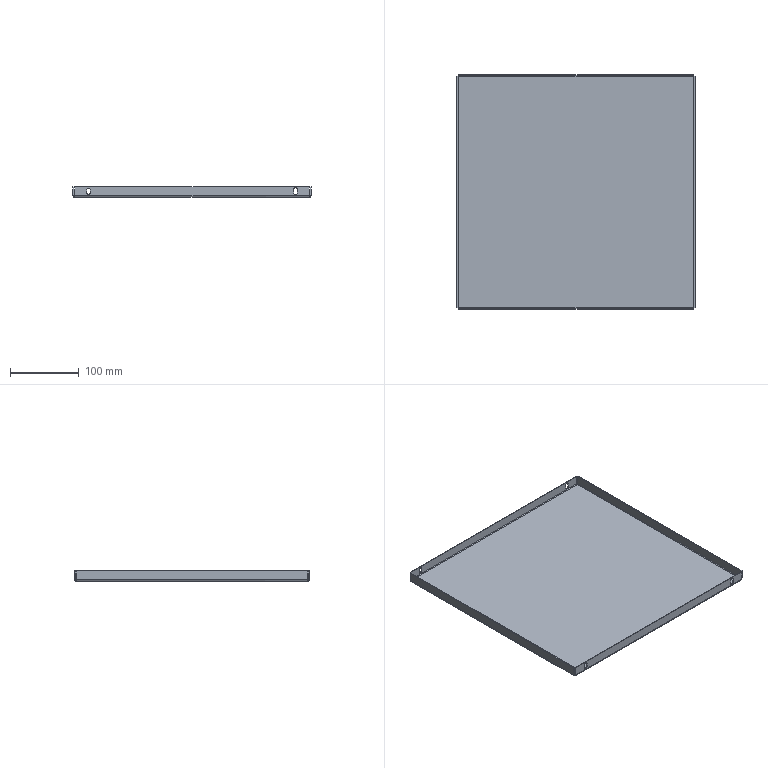Part | NX | features BREP 1 | 1 solid | 54 faces | box 345 x 340 x 15 mm | volume 201720 mm3 | plane 30 | cylinder 16 | spline 8 | commonest cylinder face diameters 5.5 x8 1.473 x4 4.473 x4